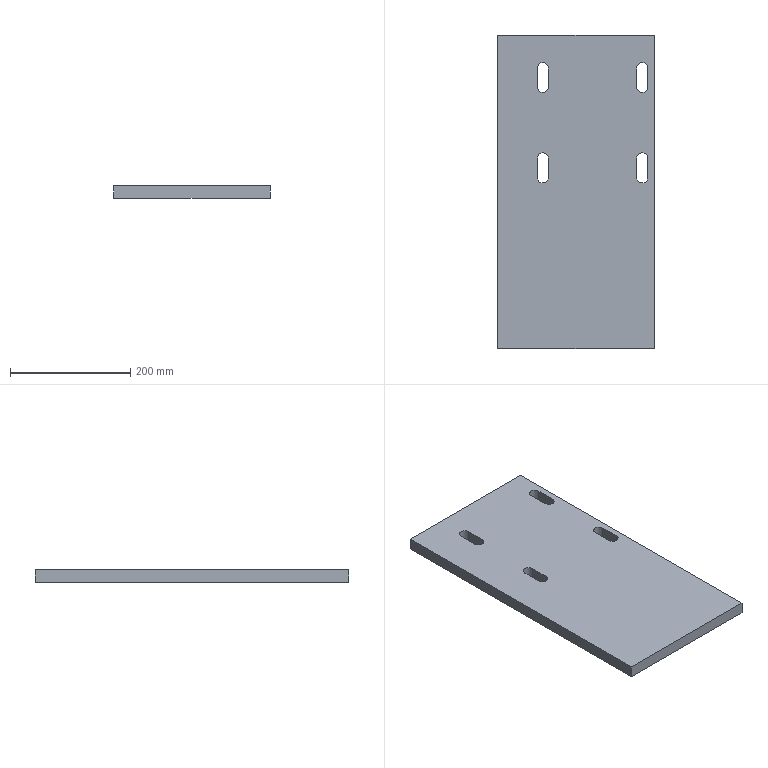Part | SolidWorks | features Extrusion 1, HoleWzd 1 | 1 solid | 22 faces | box 260 x 520 x 20 mm | volume 2637562 mm3 | plane 14 | cylinder 8 | commonest cylinder face diameters 18 x8
STEP:
#1=CARTESIAN_POINT('',(249.,284.,10.));
#2=VERTEX_POINT('',#1);
#3=CARTESIAN_POINT('',(249.,316.,10.));
#4=VERTEX_POINT('',#3);
#5=CARTESIAN_POINT('',(249.,284.,10.));
#6=DIRECTION('',(0.,1.,0.));
#7=VECTOR('',#6,1000.);
#8=LINE('',#5,#7);
#9=EDGE_CURVE('',#2,#4,#8,.T.);
#10=ORIENTED_EDGE('',*,*,#9,.F.);
#11=CARTESIAN_POINT('',(231.,284.,10.));
#12=VERTEX_POINT('',#11);
#13=CARTESIAN_POINT('',(240.,284.,10.));
#14=DIRECTION('',(0.,0.,1.));
#15=DIRECTION('',(1.,0.,0.));
#16=AXIS2_PLACEMENT_3D('',#13,#14,#15);
#17=CIRCLE('',#16,9.);
#18=EDGE_CURVE('',#12,#2,#17,.T.);
#19=ORIENTED_EDGE('',*,*,#18,.F.);
#20=CARTESIAN_POINT('',(231.,316.,10.));
#21=VERTEX_POINT('',#20);
#22=CARTESIAN_POINT('',(231.,284.,10.));
#23=DIRECTION('',(0.,1.,0.));
#24=VECTOR('',#23,1000.);
#25=LINE('',#22,#24);
#26=EDGE_CURVE('',#12,#21,#25,.T.);
#27=ORIENTED_EDGE('',*,*,#26,.T.);
#28=CARTESIAN_POINT('',(240.,316.,10.));
#29=DIRECTION('',(0.,0.,1.));
#30=DIRECTION('',(1.,0.,0.));
#31=AXIS2_PLACEMENT_3D('',#28,#29,#30);
#32=CIRCLE('',#31,9.);
#33=EDGE_CURVE('',#4,#21,#32,.T.);
#34=ORIENTED_EDGE('',*,*,#33,.F.);
#35=EDGE_LOOP('',(#10,#19,#27,#34));
#36=FACE_BOUND('',#35,.T.);
#37=CARTESIAN_POINT('',(231.,434.,10.));
#38=VERTEX_POINT('',#37);
#39=CARTESIAN_POINT('',(231.,466.,10.));
#40=VERTEX_POINT('',#39);
#41=CARTESIAN_POINT('',(231.,434.,10.));
#42=DIRECTION('',(0.,1.,0.));
#43=VECTOR('',#42,1000.);
#44=LINE('',#41,#43);
#45=EDGE_CURVE('',#38,#40,#44,.T.);
#46=ORIENTED_EDGE('',*,*,#45,.T.);
#47=CARTESIAN_POINT('',(249.,466.,10.));
#48=VERTEX_POINT('',#47);
#49=CARTESIAN_POINT('',(240.,466.,10.));
#50=DIRECTION('',(0.,0.,1.));
#51=DIRECTION('',(1.,0.,0.));
#52=AXIS2_PLACEMENT_3D('',#49,#50,#51);
#53=CIRCLE('',#52,9.);
#54=EDGE_CURVE('',#48,#40,#53,.T.);
#55=ORIENTED_EDGE('',*,*,#54,.F.);
#56=CARTESIAN_POINT('',(249.,434.,10.));
#57=VERTEX_POINT('',#56);
#58=CARTESIAN_POINT('',(249.,434.,10.));
#59=DIRECTION('',(0.,1.,0.));
#60=VECTOR('',#59,1000.);
#61=LINE('',#58,#60);
#62=EDGE_CURVE('',#57,#48,#61,.T.);
#63=ORIENTED_EDGE('',*,*,#62,.F.);
#64=CARTESIAN_POINT('',(240.,434.,10.));
#65=DIRECTION('',(0.,0.,1.));
#66=DIRECTION('',(1.,0.,0.));
#67=AXIS2_PLACEMENT_3D('',#64,#65,#66);
#68=CIRCLE('',#67,9.);
#69=EDGE_CURVE('',#38,#57,#68,.T.);
#70=ORIENTED_EDGE('',*,*,#69,.F.);
#71=EDGE_LOOP('',(#46,#55,#63,#70));
#72=FACE_BOUND('',#71,.T.);
#73=CARTESIAN_POINT('',(0.,520.,10.));
#74=VERTEX_POINT('',#73);
#75=CARTESIAN_POINT('',(0.,0.,10.));
#76=VERTEX_POINT('',#75);
#77=CARTESIAN_POINT('',(0.,0.,10.));
#78=DIRECTION('',(0.,-1.,0.));
#79=VECTOR('',#78,1000.);
#80=LINE('',#77,#79);
#81=EDGE_CURVE('',#74,#76,#80,.T.);
#82=ORIENTED_EDGE('',*,*,#81,.T.);
#83=CARTESIAN_POINT('',(260.,0.,10.));
#84=VERTEX_POINT('',#83);
#85=CARTESIAN_POINT('',(0.,0.,10.));
#86=DIRECTION('',(1.,0.,0.));
#87=VECTOR('',#86,1000.);
#88=LINE('',#85,#87);
#89=EDGE_CURVE('',#76,#84,#88,.T.);
#90=ORIENTED_EDGE('',*,*,#89,.T.);
#91=CARTESIAN_POINT('',(260.,520.,10.));
#92=VERTEX_POINT('',#91);
#93=CARTESIAN_POINT('',(260.,0.,10.));
#94=DIRECTION('',(0.,1.,0.));
#95=VECTOR('',#94,1000.);
#96=LINE('',#93,#95);
#97=EDGE_CURVE('',#84,#92,#96,.T.);
#98=ORIENTED_EDGE('',*,*,#97,.T.);
#99=CARTESIAN_POINT('',(0.,520.,10.));
#100=DIRECTION('',(-1.,0.,0.));
#101=VECTOR('',#100,1000.);
#102=LINE('',#99,#101);
#103=EDGE_CURVE('',#92,#74,#102,.T.);
#104=ORIENTED_EDGE('',*,*,#103,.T.);
#105=EDGE_LOOP('',(#82,#90,#98,#104));
#106=FACE_OUTER_BOUND('',#105,.T.);
#107=CARTESIAN_POINT('',(84.,434.,10.));
#108=VERTEX_POINT('',#107);
#109=CARTESIAN_POINT('',(84.,466.,10.));
#110=VERTEX_POINT('',#109);
#111=CARTESIAN_POINT('',(84.,434.,10.));
#112=DIRECTION('',(0.,1.,0.));
#113=VECTOR('',#112,1000.);
#114=LINE('',#111,#113);
#115=EDGE_CURVE('',#108,#110,#114,.T.);
#116=ORIENTED_EDGE('',*,*,#115,.F.);
#117=CARTESIAN_POINT('',(66.,434.,10.));
#118=VERTEX_POINT('',#117);
#119=CARTESIAN_POINT('',(75.,434.,10.));
#120=DIRECTION('',(0.,0.,1.));
#121=DIRECTION('',(1.,0.,0.));
#122=AXIS2_PLACEMENT_3D('',#119,#120,#121);
#123=CIRCLE('',#122,9.);
#124=EDGE_CURVE('',#118,#108,#123,.T.);
#125=ORIENTED_EDGE('',*,*,#124,.F.);
#126=CARTESIAN_POINT('',(66.,466.,10.));
#127=VERTEX_POINT('',#126);
#128=CARTESIAN_POINT('',(66.,434.,10.));
#129=DIRECTION('',(0.,1.,0.));
#130=VECTOR('',#129,1000.);
#131=LINE('',#128,#130);
#132=EDGE_CURVE('',#118,#127,#131,.T.);
#133=ORIENTED_EDGE('',*,*,#132,.T.);
#134=CARTESIAN_POINT('',(75.,466.,10.));
#135=DIRECTION('',(0.,0.,1.));
#136=DIRECTION('',(1.,0.,0.));
#137=AXIS2_PLACEMENT_3D('',#134,#135,#136);
#138=CIRCLE('',#137,9.);
#139=EDGE_CURVE('',#110,#127,#138,.T.);
#140=ORIENTED_EDGE('',*,*,#139,.F.);
#141=EDGE_LOOP('',(#116,#125,#133,#140));
#142=FACE_BOUND('',#141,.T.);
#143=CARTESIAN_POINT('',(84.,284.,10.));
#144=VERTEX_POINT('',#143);
#145=CARTESIAN_POINT('',(84.,316.,10.));
#146=VERTEX_POINT('',#145);
#147=CARTESIAN_POINT('',(84.,284.,10.));
#148=DIRECTION('',(0.,1.,0.));
#149=VECTOR('',#148,1000.);
#150=LINE('',#147,#149);
#151=EDGE_CURVE('',#144,#146,#150,.T.);
#152=ORIENTED_EDGE('',*,*,#151,.F.);
#153=CARTESIAN_POINT('',(66.,284.,10.));
#154=VERTEX_POINT('',#153);
#155=CARTESIAN_POINT('',(75.,284.,10.));
#156=DIRECTION('',(0.,0.,1.));
#157=DIRECTION('',(1.,0.,0.));
#158=AXIS2_PLACEMENT_3D('',#155,#156,#157);
#159=CIRCLE('',#158,9.);
#160=EDGE_CURVE('',#154,#144,#159,.T.);
#161=ORIENTED_EDGE('',*,*,#160,.F.);
#162=CARTESIAN_POINT('',(66.,316.,10.));
#163=VERTEX_POINT('',#162);
#164=CARTESIAN_POINT('',(66.,284.,10.));
#165=DIRECTION('',(0.,1.,0.));
#166=VECTOR('',#165,1000.);
#167=LINE('',#164,#166);
#168=EDGE_CURVE('',#154,#163,#167,.T.);
#169=ORIENTED_EDGE('',*,*,#168,.T.);
#170=CARTESIAN_POINT('',(75.,316.,10.));
#171=DIRECTION('',(0.,0.,1.));
#172=DIRECTION('',(1.,0.,0.));
#173=AXIS2_PLACEMENT_3D('',#170,#171,#172);
#174=CIRCLE('',#173,9.);
#175=EDGE_CURVE('',#146,#163,#174,.T.);
#176=ORIENTED_EDGE('',*,*,#175,.F.);
#177=EDGE_LOOP('',(#152,#161,#169,#176));
#178=FACE_BOUND('',#177,.T.);
#179=CARTESIAN_POINT('',(0.,0.,10.));
#180=DIRECTION('',(0.,0.,-1.));
#181=DIRECTION('',(-1.,0.,0.));
#182=AXIS2_PLACEMENT_3D('',#179,#180,#181);
#183=PLANE('',#182);
#184=ADVANCED_FACE('',(#36,#72,#106,#142,#178),#183,.F.);
#185=CARTESIAN_POINT('',(0.,520.,-10.));
#186=VERTEX_POINT('',#185);
#187=CARTESIAN_POINT('',(0.,0.,-10.));
#188=VERTEX_POINT('',#187);
#189=CARTESIAN_POINT('',(0.,0.,-10.));
#190=DIRECTION('',(0.,-1.,0.));
#191=VECTOR('',#190,1000.);
#192=LINE('',#189,#191);
#193=EDGE_CURVE('',#186,#188,#192,.T.);
#194=ORIENTED_EDGE('',*,*,#193,.T.);
#195=CARTESIAN_POINT('',(0.,0.,10.));
#196=DIRECTION('',(0.,0.,-1.));
#197=VECTOR('',#196,1000.);
#198=LINE('',#195,#197);
#199=EDGE_CURVE('',#76,#188,#198,.T.);
#200=ORIENTED_EDGE('',*,*,#199,.F.);
#201=ORIENTED_EDGE('',*,*,#81,.F.);
#202=CARTESIAN_POINT('',(0.,520.,10.));
#203=DIRECTION('',(0.,0.,-1.));
#204=VECTOR('',#203,1000.);
#205=LINE('',#202,#204);
#206=EDGE_CURVE('',#74,#186,#205,.T.);
#207=ORIENTED_EDGE('',*,*,#206,.T.);
#208=EDGE_LOOP('',(#194,#200,#201,#207));
#209=FACE_OUTER_BOUND('',#208,.T.);
#210=CARTESIAN_POINT('',(0.,0.,10.));
#211=DIRECTION('',(1.,0.,0.));
#212=DIRECTION('',(0.,0.,-1.));
#213=AXIS2_PLACEMENT_3D('',#210,#211,#212);
#214=PLANE('',#213);
#215=ADVANCED_FACE('',(#209),#214,.F.);
#216=CARTESIAN_POINT('',(260.,0.,-10.));
#217=VERTEX_POINT('',#216);
#218=CARTESIAN_POINT('',(0.,0.,-10.));
#219=DIRECTION('',(1.,0.,0.));
#220=VECTOR('',#219,1000.);
#221=LINE('',#218,#220);
#222=EDGE_CURVE('',#188,#217,#221,.T.);
#223=ORIENTED_EDGE('',*,*,#222,.T.);
#224=CARTESIAN_POINT('',(260.,0.,10.));
#225=DIRECTION('',(0.,0.,-1.));
#226=VECTOR('',#225,1000.);
#227=LINE('',#224,#226);
#228=EDGE_CURVE('',#84,#217,#227,.T.);
#229=ORIENTED_EDGE('',*,*,#228,.F.);
#230=ORIENTED_EDGE('',*,*,#89,.F.);
#231=ORIENTED_EDGE('',*,*,#199,.T.);
#232=EDGE_LOOP('',(#223,#229,#230,#231));
#233=FACE_OUTER_BOUND('',#232,.T.);
#234=CARTESIAN_POINT('',(0.,0.,10.));
#235=DIRECTION('',(0.,1.,0.));
#236=DIRECTION('',(0.,0.,1.));
#237=AXIS2_PLACEMENT_3D('',#234,#235,#236);
#238=PLANE('',#237);
#239=ADVANCED_FACE('',(#233),#238,.F.);
#240=CARTESIAN_POINT('',(260.,520.,-10.));
#241=VERTEX_POINT('',#240);
#242=CARTESIAN_POINT('',(260.,0.,-10.));
#243=DIRECTION('',(0.,1.,0.));
#244=VECTOR('',#243,1000.);
#245=LINE('',#242,#244);
#246=EDGE_CURVE('',#217,#241,#245,.T.);
#247=ORIENTED_EDGE('',*,*,#246,.T.);
#248=CARTESIAN_POINT('',(260.,520.,10.));
#249=DIRECTION('',(0.,0.,-1.));
#250=VECTOR('',#249,1000.);
#251=LINE('',#248,#250);
#252=EDGE_CURVE('',#92,#241,#251,.T.);
#253=ORIENTED_EDGE('',*,*,#252,.F.);
#254=ORIENTED_EDGE('',*,*,#97,.F.);
#255=ORIENTED_EDGE('',*,*,#228,.T.);
#256=EDGE_LOOP('',(#247,#253,#254,#255));
#257=FACE_OUTER_BOUND('',#256,.T.);
#258=CARTESIAN_POINT('',(260.,0.,10.));
#259=DIRECTION('',(-1.,0.,0.));
#260=DIRECTION('',(0.,0.,1.));
#261=AXIS2_PLACEMENT_3D('',#258,#259,#260);
#262=PLANE('',#261);
#263=ADVANCED_FACE('',(#257),#262,.F.);
#264=CARTESIAN_POINT('',(0.,520.,-10.));
#265=DIRECTION('',(-1.,0.,0.));
#266=VECTOR('',#265,1000.);
#267=LINE('',#264,#266);
#268=EDGE_CURVE('',#241,#186,#267,.T.);
#269=ORIENTED_EDGE('',*,*,#268,.T.);
#270=ORIENTED_EDGE('',*,*,#206,.F.);
#271=ORIENTED_EDGE('',*,*,#103,.F.);
#272=ORIENTED_EDGE('',*,*,#252,.T.);
#273=EDGE_LOOP('',(#269,#270,#271,#272));
#274=FACE_OUTER_BOUND('',#273,.T.);
#275=CARTESIAN_POINT('',(0.,520.,10.));
#276=DIRECTION('',(0.,-1.,0.));
#277=DIRECTION('',(0.,0.,-1.));
#278=AXIS2_PLACEMENT_3D('',#275,#276,#277);
#279=PLANE('',#278);
#280=ADVANCED_FACE('',(#274),#279,.F.);
#281=CARTESIAN_POINT('',(66.,284.,-10.));
#282=VERTEX_POINT('',#281);
#283=CARTESIAN_POINT('',(66.,316.,-10.));
#284=VERTEX_POINT('',#283);
#285=CARTESIAN_POINT('',(66.,0.,-10.));
#286=DIRECTION('',(0.,1.,0.));
#287=VECTOR('',#286,1000.);
#288=LINE('',#285,#287);
#289=EDGE_CURVE('',#282,#284,#288,.T.);
#290=ORIENTED_EDGE('',*,*,#289,.F.);
#291=CARTESIAN_POINT('',(84.,284.,-10.));
#292=VERTEX_POINT('',#291);
#293=CARTESIAN_POINT('',(75.,284.,-10.));
#294=DIRECTION('',(0.,0.,-1.));
#295=DIRECTION('',(-1.,0.,0.));
#296=AXIS2_PLACEMENT_3D('',#293,#294,#295);
#297=CIRCLE('',#296,9.);
#298=EDGE_CURVE('',#292,#282,#297,.T.);
#299=ORIENTED_EDGE('',*,*,#298,.F.);
#300=CARTESIAN_POINT('',(84.,316.,-10.));
#301=VERTEX_POINT('',#300);
#302=CARTESIAN_POINT('',(84.,0.,-10.));
#303=DIRECTION('',(0.,-1.,0.));
#304=VECTOR('',#303,1000.);
#305=LINE('',#302,#304);
#306=EDGE_CURVE('',#301,#292,#305,.T.);
#307=ORIENTED_EDGE('',*,*,#306,.F.);
#308=CARTESIAN_POINT('',(75.,316.,-10.));
#309=DIRECTION('',(0.,0.,-1.));
#310=DIRECTION('',(-1.,0.,0.));
#311=AXIS2_PLACEMENT_3D('',#308,#309,#310);
#312=CIRCLE('',#311,9.);
#313=EDGE_CURVE('',#284,#301,#312,.T.);
#314=ORIENTED_EDGE('',*,*,#313,.F.);
#315=EDGE_LOOP('',(#290,#299,#307,#314));
#316=FACE_BOUND('',#315,.T.);
#317=CARTESIAN_POINT('',(231.,284.,-10.));
#318=VERTEX_POINT('',#317);
#319=CARTESIAN_POINT('',(231.,316.,-10.));
#320=VERTEX_POINT('',#319);
#321=CARTESIAN_POINT('',(231.,0.,-10.));
#322=DIRECTION('',(0.,1.,0.));
#323=VECTOR('',#322,1000.);
#324=LINE('',#321,#323);
#325=EDGE_CURVE('',#318,#320,#324,.T.);
#326=ORIENTED_EDGE('',*,*,#325,.F.);
#327=CARTESIAN_POINT('',(249.,284.,-10.));
#328=VERTEX_POINT('',#327);
#329=CARTESIAN_POINT('',(240.,284.,-10.));
#330=DIRECTION('',(0.,0.,-1.));
#331=DIRECTION('',(-1.,0.,0.));
#332=AXIS2_PLACEMENT_3D('',#329,#330,#331);
#333=CIRCLE('',#332,9.);
#334=EDGE_CURVE('',#328,#318,#333,.T.);
#335=ORIENTED_EDGE('',*,*,#334,.F.);
#336=CARTESIAN_POINT('',(249.,316.,-10.));
#337=VERTEX_POINT('',#336);
#338=CARTESIAN_POINT('',(249.,0.,-10.));
#339=DIRECTION('',(0.,-1.,0.));
#340=VECTOR('',#339,1000.);
#341=LINE('',#338,#340);
#342=EDGE_CURVE('',#337,#328,#341,.T.);
#343=ORIENTED_EDGE('',*,*,#342,.F.);
#344=CARTESIAN_POINT('',(240.,316.,-10.));
#345=DIRECTION('',(0.,0.,-1.));
#346=DIRECTION('',(-1.,0.,0.));
#347=AXIS2_PLACEMENT_3D('',#344,#345,#346);
#348=CIRCLE('',#347,9.);
#349=EDGE_CURVE('',#320,#337,#348,.T.);
#350=ORIENTED_EDGE('',*,*,#349,.F.);
#351=EDGE_LOOP('',(#326,#335,#343,#350));
#352=FACE_BOUND('',#351,.T.);
#353=CARTESIAN_POINT('',(231.,434.,-10.));
#354=VERTEX_POINT('',#353);
#355=CARTESIAN_POINT('',(231.,466.,-10.));
#356=VERTEX_POINT('',#355);
#357=CARTESIAN_POINT('',(231.,0.,-10.));
#358=DIRECTION('',(0.,1.,0.));
#359=VECTOR('',#358,1000.);
#360=LINE('',#357,#359);
#361=EDGE_CURVE('',#354,#356,#360,.T.);
#362=ORIENTED_EDGE('',*,*,#361,.F.);
#363=CARTESIAN_POINT('',(249.,434.,-10.));
#364=VERTEX_POINT('',#363);
#365=CARTESIAN_POINT('',(240.,434.,-10.));
#366=DIRECTION('',(0.,0.,-1.));
#367=DIRECTION('',(-1.,0.,0.));
#368=AXIS2_PLACEMENT_3D('',#365,#366,#367);
#369=CIRCLE('',#368,9.);
#370=EDGE_CURVE('',#364,#354,#369,.T.);
#371=ORIENTED_EDGE('',*,*,#370,.F.);
#372=CARTESIAN_POINT('',(249.,466.,-10.));
#373=VERTEX_POINT('',#372);
#374=CARTESIAN_POINT('',(249.,0.,-10.));
#375=DIRECTION('',(0.,-1.,0.));
#376=VECTOR('',#375,1000.);
#377=LINE('',#374,#376);
#378=EDGE_CURVE('',#373,#364,#377,.T.);
#379=ORIENTED_EDGE('',*,*,#378,.F.);
#380=CARTESIAN_POINT('',(240.,466.,-10.));
#381=DIRECTION('',(0.,0.,-1.));
#382=DIRECTION('',(-1.,0.,0.));
#383=AXIS2_PLACEMENT_3D('',#380,#381,#382);
#384=CIRCLE('',#383,9.);
#385=EDGE_CURVE('',#356,#373,#384,.T.);
#386=ORIENTED_EDGE('',*,*,#385,.F.);
#387=EDGE_LOOP('',(#362,#371,#379,#386));
#388=FACE_BOUND('',#387,.T.);
#389=CARTESIAN_POINT('',(66.,434.,-10.));
#390=VERTEX_POINT('',#389);
#391=CARTESIAN_POINT('',(66.,466.,-10.));
#392=VERTEX_POINT('',#391);
#393=CARTESIAN_POINT('',(66.,0.,-10.));
#394=DIRECTION('',(0.,1.,0.));
#395=VECTOR('',#394,1000.);
#396=LINE('',#393,#395);
#397=EDGE_CURVE('',#390,#392,#396,.T.);
#398=ORIENTED_EDGE('',*,*,#397,.F.);
#399=CARTESIAN_POINT('',(84.,434.,-10.));
#400=VERTEX_POINT('',#399);
#401=CARTESIAN_POINT('',(75.,434.,-10.));
#402=DIRECTION('',(0.,0.,-1.));
#403=DIRECTION('',(-1.,0.,0.));
#404=AXIS2_PLACEMENT_3D('',#401,#402,#403);
#405=CIRCLE('',#404,9.);
#406=EDGE_CURVE('',#400,#390,#405,.T.);
#407=ORIENTED_EDGE('',*,*,#406,.F.);
#408=CARTESIAN_POINT('',(84.,466.,-10.));
#409=VERTEX_POINT('',#408);
#410=CARTESIAN_POINT('',(84.,0.,-10.));
#411=DIRECTION('',(0.,-1.,0.));
#412=VECTOR('',#411,1000.);
#413=LINE('',#410,#412);
#414=EDGE_CURVE('',#409,#400,#413,.T.);
#415=ORIENTED_EDGE('',*,*,#414,.F.);
#416=CARTESIAN_POINT('',(75.,466.,-10.));
#417=DIRECTION('',(0.,0.,-1.));
#418=DIRECTION('',(-1.,0.,0.));
#419=AXIS2_PLACEMENT_3D('',#416,#417,#418);
#420=CIRCLE('',#419,9.);
#421=EDGE_CURVE('',#392,#409,#420,.T.);
#422=ORIENTED_EDGE('',*,*,#421,.F.);
#423=EDGE_LOOP('',(#398,#407,#415,#422));
#424=FACE_BOUND('',#423,.T.);
#425=ORIENTED_EDGE('',*,*,#193,.F.);
#426=ORIENTED_EDGE('',*,*,#268,.F.);
#427=ORIENTED_EDGE('',*,*,#246,.F.);
#428=ORIENTED_EDGE('',*,*,#222,.F.);
#429=EDGE_LOOP('',(#425,#426,#427,#428));
#430=FACE_OUTER_BOUND('',#429,.T.);
#431=CARTESIAN_POINT('',(0.,0.,-10.));
#432=DIRECTION('',(0.,0.,-1.));
#433=DIRECTION('',(-1.,0.,0.));
#434=AXIS2_PLACEMENT_3D('',#431,#432,#433);
#435=PLANE('',#434);
#436=ADVANCED_FACE('',(#316,#352,#388,#424,#430),#435,.T.);
#437=ORIENTED_EDGE('',*,*,#421,.T.);
#438=CARTESIAN_POINT('',(84.,466.,-10.001));
#439=DIRECTION('',(0.,0.,-1.));
#440=VECTOR('',#439,1000.);
#441=LINE('',#438,#440);
#442=EDGE_CURVE('',#110,#409,#441,.T.);
#443=ORIENTED_EDGE('',*,*,#442,.F.);
#444=ORIENTED_EDGE('',*,*,#139,.T.);
#445=CARTESIAN_POINT('',(66.,466.,10.));
#446=DIRECTION('',(0.,0.,1.));
#447=VECTOR('',#446,1000.);
#448=LINE('',#445,#447);
#449=EDGE_CURVE('',#392,#127,#448,.T.);
#450=ORIENTED_EDGE('',*,*,#449,.F.);
#451=EDGE_LOOP('',(#437,#443,#444,#450));
#452=FACE_OUTER_BOUND('',#451,.T.);
#453=CARTESIAN_POINT('',(75.,466.,10.));
#454=DIRECTION('',(0.,0.,1.));
#455=DIRECTION('',(1.,0.,0.));
#456=AXIS2_PLACEMENT_3D('',#453,#454,#455);
#457=CYLINDRICAL_SURFACE('',#456,9.);
#458=ADVANCED_FACE('',(#452),#457,.F.);
#459=ORIENTED_EDGE('',*,*,#406,.T.);
#460=CARTESIAN_POINT('',(66.,434.,10.));
#461=DIRECTION('',(0.,0.,-1.));
#462=VECTOR('',#461,1000.);
#463=LINE('',#460,#462);
#464=EDGE_CURVE('',#118,#390,#463,.T.);
#465=ORIENTED_EDGE('',*,*,#464,.F.);
#466=ORIENTED_EDGE('',*,*,#124,.T.);
#467=CARTESIAN_POINT('',(84.,434.,-10.001));
#468=DIRECTION('',(0.,0.,-1.));
#469=VECTOR('',#468,1000.);
#470=LINE('',#467,#469);
#471=EDGE_CURVE('',#108,#400,#470,.T.);
#472=ORIENTED_EDGE('',*,*,#471,.T.);
#473=EDGE_LOOP('',(#459,#465,#466,#472));
#474=FACE_OUTER_BOUND('',#473,.T.);
#475=CARTESIAN_POINT('',(75.,434.,10.));
#476=DIRECTION('',(0.,0.,1.));
#477=DIRECTION('',(1.,0.,0.));
#478=AXIS2_PLACEMENT_3D('',#475,#476,#477);
#479=CYLINDRICAL_SURFACE('',#478,9.);
#480=ADVANCED_FACE('',(#474),#479,.F.);
#481=ORIENTED_EDGE('',*,*,#397,.T.);
#482=ORIENTED_EDGE('',*,*,#449,.T.);
#483=ORIENTED_EDGE('',*,*,#132,.F.);
#484=ORIENTED_EDGE('',*,*,#464,.T.);
#485=EDGE_LOOP('',(#481,#482,#483,#484));
#486=FACE_OUTER_BOUND('',#485,.T.);
#487=CARTESIAN_POINT('',(66.,434.,10.));
#488=DIRECTION('',(-1.,0.,0.));
#489=DIRECTION('',(0.,0.,1.));
#490=AXIS2_PLACEMENT_3D('',#487,#488,#489);
#491=PLANE('',#490);
#492=ADVANCED_FACE('',(#486),#491,.F.);
#493=ORIENTED_EDGE('',*,*,#414,.T.);
#494=ORIENTED_EDGE('',*,*,#471,.F.);
#495=ORIENTED_EDGE('',*,*,#115,.T.);
#496=ORIENTED_EDGE('',*,*,#442,.T.);
#497=EDGE_LOOP('',(#493,#494,#495,#496));
#498=FACE_OUTER_BOUND('',#497,.T.);
#499=CARTESIAN_POINT('',(84.,434.,-10.001));
#500=DIRECTION('',(1.,0.,0.));
#501=DIRECTION('',(0.,0.,-1.));
#502=AXIS2_PLACEMENT_3D('',#499,#500,#501);
#503=PLANE('',#502);
#504=ADVANCED_FACE('',(#498),#503,.F.);
#505=ORIENTED_EDGE('',*,*,#385,.T.);
#506=CARTESIAN_POINT('',(249.,466.,-10.001));
#507=DIRECTION('',(0.,0.,-1.));
#508=VECTOR('',#507,1000.);
#509=LINE('',#506,#508);
#510=EDGE_CURVE('',#48,#373,#509,.T.);
#511=ORIENTED_EDGE('',*,*,#510,.F.);
#512=ORIENTED_EDGE('',*,*,#54,.T.);
#513=CARTESIAN_POINT('',(231.,466.,10.));
#514=DIRECTION('',(0.,0.,1.));
#515=VECTOR('',#514,1000.);
#516=LINE('',#513,#515);
#517=EDGE_CURVE('',#356,#40,#516,.T.);
#518=ORIENTED_EDGE('',*,*,#517,.F.);
#519=EDGE_LOOP('',(#505,#511,#512,#518));
#520=FACE_OUTER_BOUND('',#519,.T.);
#521=CARTESIAN_POINT('',(240.,466.,10.));
#522=DIRECTION('',(0.,0.,1.));
#523=DIRECTION('',(1.,0.,0.));
#524=AXIS2_PLACEMENT_3D('',#521,#522,#523);
#525=CYLINDRICAL_SURFACE('',#524,9.);
#526=ADVANCED_FACE('',(#520),#525,.F.);
#527=ORIENTED_EDGE('',*,*,#370,.T.);
#528=CARTESIAN_POINT('',(231.,434.,10.));
#529=DIRECTION('',(0.,0.,-1.));
#530=VECTOR('',#529,1000.);
#531=LINE('',#528,#530);
#532=EDGE_CURVE('',#38,#354,#531,.T.);
#533=ORIENTED_EDGE('',*,*,#532,.F.);
#534=ORIENTED_EDGE('',*,*,#69,.T.);
#535=CARTESIAN_POINT('',(249.,434.,-10.001));
#536=DIRECTION('',(0.,0.,-1.));
#537=VECTOR('',#536,1000.);
#538=LINE('',#535,#537);
#539=EDGE_CURVE('',#57,#364,#538,.T.);
#540=ORIENTED_EDGE('',*,*,#539,.T.);
#541=EDGE_LOOP('',(#527,#533,#534,#540));
#542=FACE_OUTER_BOUND('',#541,.T.);
#543=CARTESIAN_POINT('',(240.,434.,10.));
#544=DIRECTION('',(0.,0.,1.));
#545=DIRECTION('',(1.,0.,0.));
#546=AXIS2_PLACEMENT_3D('',#543,#544,#545);
#547=CYLINDRICAL_SURFACE('',#546,9.);
#548=ADVANCED_FACE('',(#542),#547,.F.);
#549=ORIENTED_EDGE('',*,*,#361,.T.);
#550=ORIENTED_EDGE('',*,*,#517,.T.);
#551=ORIENTED_EDGE('',*,*,#45,.F.);
#552=ORIENTED_EDGE('',*,*,#532,.T.);
#553=EDGE_LOOP('',(#549,#550,#551,#552));
#554=FACE_OUTER_BOUND('',#553,.T.);
#555=CARTESIAN_POINT('',(231.,434.,10.));
#556=DIRECTION('',(-1.,0.,0.));
#557=DIRECTION('',(0.,0.,1.));
#558=AXIS2_PLACEMENT_3D('',#555,#556,#557);
#559=PLANE('',#558);
#560=ADVANCED_FACE('',(#554),#559,.F.);
#561=ORIENTED_EDGE('',*,*,#378,.T.);
#562=ORIENTED_EDGE('',*,*,#539,.F.);
#563=ORIENTED_EDGE('',*,*,#62,.T.);
#564=ORIENTED_EDGE('',*,*,#510,.T.);
#565=EDGE_LOOP('',(#561,#562,#563,#564));
#566=FACE_OUTER_BOUND('',#565,.T.);
#567=CARTESIAN_POINT('',(249.,434.,-10.001));
#568=DIRECTION('',(1.,0.,0.));
#569=DIRECTION('',(0.,0.,-1.));
#570=AXIS2_PLACEMENT_3D('',#567,#568,#569);
#571=PLANE('',#570);
#572=ADVANCED_FACE('',(#566),#571,.F.);
#573=ORIENTED_EDGE('',*,*,#349,.T.);
#574=CARTESIAN_POINT('',(249.,316.,-10.001));
#575=DIRECTION('',(0.,0.,-1.));
#576=VECTOR('',#575,1000.);
#577=LINE('',#574,#576);
#578=EDGE_CURVE('',#4,#337,#577,.T.);
#579=ORIENTED_EDGE('',*,*,#578,.F.);
#580=ORIENTED_EDGE('',*,*,#33,.T.);
#581=CARTESIAN_POINT('',(231.,316.,10.));
#582=DIRECTION('',(0.,0.,1.));
#583=VECTOR('',#582,1000.);
#584=LINE('',#581,#583);
#585=EDGE_CURVE('',#320,#21,#584,.T.);
#586=ORIENTED_EDGE('',*,*,#585,.F.);
#587=EDGE_LOOP('',(#573,#579,#580,#586));
#588=FACE_OUTER_BOUND('',#587,.T.);
#589=CARTESIAN_POINT('',(240.,316.,10.));
#590=DIRECTION('',(0.,0.,1.));
#591=DIRECTION('',(1.,0.,0.));
#592=AXIS2_PLACEMENT_3D('',#589,#590,#591);
#593=CYLINDRICAL_SURFACE('',#592,9.);
#594=ADVANCED_FACE('',(#588),#593,.F.);
#595=ORIENTED_EDGE('',*,*,#334,.T.);
#596=CARTESIAN_POINT('',(231.,284.,10.));
#597=DIRECTION('',(0.,0.,-1.));
#598=VECTOR('',#597,1000.);
#599=LINE('',#596,#598);
#600=EDGE_CURVE('',#12,#318,#599,.T.);
#601=ORIENTED_EDGE('',*,*,#600,.F.);
#602=ORIENTED_EDGE('',*,*,#18,.T.);
#603=CARTESIAN_POINT('',(249.,284.,-10.001));
#604=DIRECTION('',(0.,0.,-1.));
#605=VECTOR('',#604,1000.);
#606=LINE('',#603,#605);
#607=EDGE_CURVE('',#2,#328,#606,.T.);
#608=ORIENTED_EDGE('',*,*,#607,.T.);
#609=EDGE_LOOP('',(#595,#601,#602,#608));
#610=FACE_OUTER_BOUND('',#609,.T.);
#611=CARTESIAN_POINT('',(240.,284.,10.));
#612=DIRECTION('',(0.,0.,1.));
#613=DIRECTION('',(1.,0.,0.));
#614=AXIS2_PLACEMENT_3D('',#611,#612,#613);
#615=CYLINDRICAL_SURFACE('',#614,9.);
#616=ADVANCED_FACE('',(#610),#615,.F.);
#617=ORIENTED_EDGE('',*,*,#325,.T.);
#618=ORIENTED_EDGE('',*,*,#585,.T.);
#619=ORIENTED_EDGE('',*,*,#26,.F.);
#620=ORIENTED_EDGE('',*,*,#600,.T.);
#621=EDGE_LOOP('',(#617,#618,#619,#620));
#622=FACE_OUTER_BOUND('',#621,.T.);
#623=CARTESIAN_POINT('',(231.,284.,10.));
#624=DIRECTION('',(-1.,0.,0.));
#625=DIRECTION('',(0.,0.,1.));
#626=AXIS2_PLACEMENT_3D('',#623,#624,#625);
#627=PLANE('',#626);
#628=ADVANCED_FACE('',(#622),#627,.F.);
#629=ORIENTED_EDGE('',*,*,#342,.T.);
#630=ORIENTED_EDGE('',*,*,#607,.F.);
#631=ORIENTED_EDGE('',*,*,#9,.T.);
#632=ORIENTED_EDGE('',*,*,#578,.T.);
#633=EDGE_LOOP('',(#629,#630,#631,#632));
#634=FACE_OUTER_BOUND('',#633,.T.);
#635=CARTESIAN_POINT('',(249.,284.,-10.001));
#636=DIRECTION('',(1.,0.,0.));
#637=DIRECTION('',(0.,0.,-1.));
#638=AXIS2_PLACEMENT_3D('',#635,#636,#637);
#639=PLANE('',#638);
#640=ADVANCED_FACE('',(#634),#639,.F.);
#641=ORIENTED_EDGE('',*,*,#313,.T.);
#642=CARTESIAN_POINT('',(84.,316.,-10.001));
#643=DIRECTION('',(0.,0.,-1.));
#644=VECTOR('',#643,1000.);
#645=LINE('',#642,#644);
#646=EDGE_CURVE('',#146,#301,#645,.T.);
#647=ORIENTED_EDGE('',*,*,#646,.F.);
#648=ORIENTED_EDGE('',*,*,#175,.T.);
#649=CARTESIAN_POINT('',(66.,316.,10.));
#650=DIRECTION('',(0.,0.,1.));
#651=VECTOR('',#650,1000.);
#652=LINE('',#649,#651);
#653=EDGE_CURVE('',#284,#163,#652,.T.);
#654=ORIENTED_EDGE('',*,*,#653,.F.);
#655=EDGE_LOOP('',(#641,#647,#648,#654));
#656=FACE_OUTER_BOUND('',#655,.T.);
#657=CARTESIAN_POINT('',(75.,316.,10.));
#658=DIRECTION('',(0.,0.,1.));
#659=DIRECTION('',(1.,0.,0.));
#660=AXIS2_PLACEMENT_3D('',#657,#658,#659);
#661=CYLINDRICAL_SURFACE('',#660,9.);
#662=ADVANCED_FACE('',(#656),#661,.F.);
#663=ORIENTED_EDGE('',*,*,#298,.T.);
#664=CARTESIAN_POINT('',(66.,284.,10.));
#665=DIRECTION('',(0.,0.,-1.));
#666=VECTOR('',#665,1000.);
#667=LINE('',#664,#666);
#668=EDGE_CURVE('',#154,#282,#667,.T.);
#669=ORIENTED_EDGE('',*,*,#668,.F.);
#670=ORIENTED_EDGE('',*,*,#160,.T.);
#671=CARTESIAN_POINT('',(84.,284.,-10.001));
#672=DIRECTION('',(0.,0.,-1.));
#673=VECTOR('',#672,1000.);
#674=LINE('',#671,#673);
#675=EDGE_CURVE('',#144,#292,#674,.T.);
#676=ORIENTED_EDGE('',*,*,#675,.T.);
#677=EDGE_LOOP('',(#663,#669,#670,#676));
#678=FACE_OUTER_BOUND('',#677,.T.);
#679=CARTESIAN_POINT('',(75.,284.,10.));
#680=DIRECTION('',(0.,0.,1.));
#681=DIRECTION('',(1.,0.,0.));
#682=AXIS2_PLACEMENT_3D('',#679,#680,#681);
#683=CYLINDRICAL_SURFACE('',#682,9.);
#684=ADVANCED_FACE('',(#678),#683,.F.);
#685=ORIENTED_EDGE('',*,*,#289,.T.);
#686=ORIENTED_EDGE('',*,*,#653,.T.);
#687=ORIENTED_EDGE('',*,*,#168,.F.);
#688=ORIENTED_EDGE('',*,*,#668,.T.);
#689=EDGE_LOOP('',(#685,#686,#687,#688));
#690=FACE_OUTER_BOUND('',#689,.T.);
#691=CARTESIAN_POINT('',(66.,284.,10.));
#692=DIRECTION('',(-1.,0.,0.));
#693=DIRECTION('',(0.,0.,1.));
#694=AXIS2_PLACEMENT_3D('',#691,#692,#693);
#695=PLANE('',#694);
#696=ADVANCED_FACE('',(#690),#695,.F.);
#697=ORIENTED_EDGE('',*,*,#306,.T.);
#698=ORIENTED_EDGE('',*,*,#675,.F.);
#699=ORIENTED_EDGE('',*,*,#151,.T.);
#700=ORIENTED_EDGE('',*,*,#646,.T.);
#701=EDGE_LOOP('',(#697,#698,#699,#700));
#702=FACE_OUTER_BOUND('',#701,.T.);
#703=CARTESIAN_POINT('',(84.,284.,-10.001));
#704=DIRECTION('',(1.,0.,0.));
#705=DIRECTION('',(0.,0.,-1.));
#706=AXIS2_PLACEMENT_3D('',#703,#704,#705);
#707=PLANE('',#706);
#708=ADVANCED_FACE('',(#702),#707,.F.);
#709=CLOSED_SHELL('',(#184,#215,#239,#263,#280,#436,#458,#480,#492,#504,#526,#548,#560,#572,#594,#616,#628,#640,#662,#684,#696,#708));
#710=MANIFOLD_SOLID_BREP('',#709);
#711=CARTESIAN_POINT('',(0.,0.,0.));
#712=DIRECTION('',(0.,0.,1.));
#713=DIRECTION('',(1.,0.,0.));
#714=AXIS2_PLACEMENT_3D('',#711,#712,#713);
#715=(LENGTH_UNIT()NAMED_UNIT(*)SI_UNIT(.MILLI.,.METRE.));
#716=UNCERTAINTY_MEASURE_WITH_UNIT(LENGTH_MEASURE(0.00001),#715,'','');
#717=(NAMED_UNIT(*)PLANE_ANGLE_UNIT()SI_UNIT($,.RADIAN.));
#718=(NAMED_UNIT(*)SI_UNIT($,.STERADIAN.)SOLID_ANGLE_UNIT());
#719=(GEOMETRIC_REPRESENTATION_CONTEXT(3)GLOBAL_UNCERTAINTY_ASSIGNED_CONTEXT((#716))GLOBAL_UNIT_ASSIGNED_CONTEXT((#715,#717,#718))REPRESENTATION_CONTEXT('',''));
#720=ADVANCED_BREP_SHAPE_REPRESENTATION('',(#710,#714),#719);